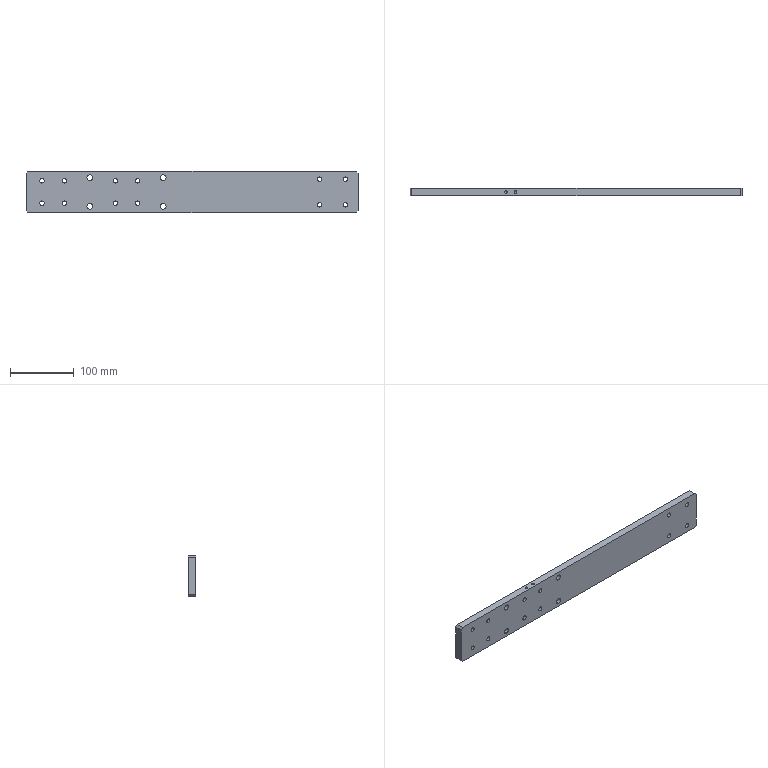Part | SolidWorks | features HoleWzd 7, Chamfer 1, Extrusion 1, LPattern 1 | 1 solid | 58 faces | box 520 x 12 x 65 mm | volume 396078 mm3 | cylinder 40 | plane 10 | cone 8 | commonest cylinder face diameters 7 x24 4.2 x8 9 x8